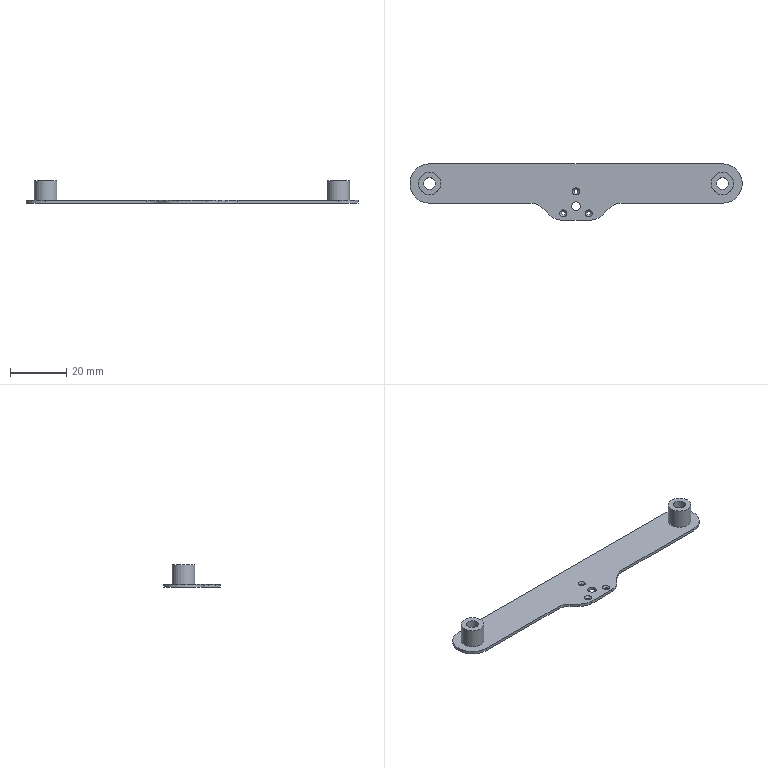Part | NX | features DATUM_CSYS 4, EXTRUDE 4, SKETCH 3, BREP 1, OFFSET_REGION 1, SCALE 1 | 1 solid | 27 faces | box 118 x 20 x 8 mm | volume 2204 mm3 | cylinder 14 | plane 10 | cone 3 | commonest cylinder face diameters 12 x4 1.32 x3 4.2 x2 8 x2 14 x2 3 x1
STEP:
#1=CARTESIAN_POINT('',(1.5,-45.,-19.5));
#2=VERTEX_POINT('',#1);
#3=CARTESIAN_POINT('',(0.,-45.,-19.5));
#4=DIRECTION('',(0.,0.,1.));
#5=DIRECTION('',(1.,0.,0.));
#6=AXIS2_PLACEMENT_3D('',#3,#4,#5);
#7=CIRCLE('',#6,1.5);
#8=EDGE_CURVE('',#2,#2,#7,.T.);
#9=ORIENTED_EDGE('',*,*,#8,.T.);
#10=EDGE_LOOP('',(#9));
#11=FACE_BOUND('',#10,.T.);
#12=CARTESIAN_POINT('',(1.5,-45.,-20.5));
#13=VERTEX_POINT('',#12);
#14=CARTESIAN_POINT('',(0.,-45.,-20.5));
#15=DIRECTION('',(0.,0.,1.));
#16=DIRECTION('',(1.,0.,0.));
#17=AXIS2_PLACEMENT_3D('',#14,#15,#16);
#18=CIRCLE('',#17,1.5);
#19=EDGE_CURVE('',#13,#13,#18,.T.);
#20=ORIENTED_EDGE('',*,*,#19,.F.);
#21=EDGE_LOOP('',(#20));
#22=FACE_BOUND('',#21,.T.);
#23=CARTESIAN_POINT('',(0.,-45.,-19.5));
#24=DIRECTION('',(0.,0.,1.));
#25=DIRECTION('',(1.,0.,0.));
#26=AXIS2_PLACEMENT_3D('',#23,#24,#25);
#27=CYLINDRICAL_SURFACE('',#26,1.5);
#28=ADVANCED_FACE('',(#11,#22),#27,.F.);
#29=CARTESIAN_POINT('',(1.26,-39.8,-19.5));
#30=VERTEX_POINT('',#29);
#31=CARTESIAN_POINT('',(0.,-39.8,-19.5));
#32=DIRECTION('',(0.,0.,1.));
#33=DIRECTION('',(1.,0.,0.));
#34=AXIS2_PLACEMENT_3D('',#31,#32,#33);
#35=CIRCLE('',#34,1.26);
#36=EDGE_CURVE('',#30,#30,#35,.T.);
#37=ORIENTED_EDGE('',*,*,#36,.T.);
#38=EDGE_LOOP('',(#37));
#39=FACE_BOUND('',#38,.T.);
#40=CARTESIAN_POINT('',(0.66,-39.8,-20.1));
#41=VERTEX_POINT('',#40);
#42=CARTESIAN_POINT('',(0.,-39.8,-20.1));
#43=DIRECTION('',(0.,0.,1.));
#44=DIRECTION('',(1.,0.,0.));
#45=AXIS2_PLACEMENT_3D('',#42,#43,#44);
#46=CIRCLE('',#45,0.66);
#47=EDGE_CURVE('',#41,#41,#46,.T.);
#48=ORIENTED_EDGE('',*,*,#47,.F.);
#49=EDGE_LOOP('',(#48));
#50=FACE_BOUND('',#49,.T.);
#51=CARTESIAN_POINT('',(0.,-39.8,-19.5));
#52=DIRECTION('',(0.,0.,1.));
#53=DIRECTION('',(1.,0.,0.));
#54=AXIS2_PLACEMENT_3D('',#51,#52,#53);
#55=CONICAL_SURFACE('',#54,1.26,0.7854);
#56=ADVANCED_FACE('',(#39,#50),#55,.F.);
#57=ORIENTED_EDGE('',*,*,#47,.T.);
#58=EDGE_LOOP('',(#57));
#59=FACE_BOUND('',#58,.T.);
#60=CARTESIAN_POINT('',(0.66,-39.8,-20.5));
#61=VERTEX_POINT('',#60);
#62=CARTESIAN_POINT('',(0.,-39.8,-20.5));
#63=DIRECTION('',(0.,0.,1.));
#64=DIRECTION('',(1.,0.,0.));
#65=AXIS2_PLACEMENT_3D('',#62,#63,#64);
#66=CIRCLE('',#65,0.66);
#67=EDGE_CURVE('',#61,#61,#66,.T.);
#68=ORIENTED_EDGE('',*,*,#67,.F.);
#69=EDGE_LOOP('',(#68));
#70=FACE_BOUND('',#69,.T.);
#71=CARTESIAN_POINT('',(0.,-39.8,-19.5));
#72=DIRECTION('',(0.,0.,1.));
#73=DIRECTION('',(1.,0.,0.));
#74=AXIS2_PLACEMENT_3D('',#71,#72,#73);
#75=CYLINDRICAL_SURFACE('',#74,0.66);
#76=ADVANCED_FACE('',(#59,#70),#75,.F.);
#77=CARTESIAN_POINT('',(-3.243,-47.6,-19.5));
#78=VERTEX_POINT('',#77);
#79=CARTESIAN_POINT('',(-4.503,-47.6,-19.5));
#80=DIRECTION('',(0.,0.,1.));
#81=DIRECTION('',(1.,0.,0.));
#82=AXIS2_PLACEMENT_3D('',#79,#80,#81);
#83=CIRCLE('',#82,1.26);
#84=EDGE_CURVE('',#78,#78,#83,.T.);
#85=ORIENTED_EDGE('',*,*,#84,.T.);
#86=EDGE_LOOP('',(#85));
#87=FACE_BOUND('',#86,.T.);
#88=CARTESIAN_POINT('',(-3.843,-47.6,-20.1));
#89=VERTEX_POINT('',#88);
#90=CARTESIAN_POINT('',(-4.503,-47.6,-20.1));
#91=DIRECTION('',(0.,0.,1.));
#92=DIRECTION('',(1.,0.,0.));
#93=AXIS2_PLACEMENT_3D('',#90,#91,#92);
#94=CIRCLE('',#93,0.66);
#95=EDGE_CURVE('',#89,#89,#94,.T.);
#96=ORIENTED_EDGE('',*,*,#95,.F.);
#97=EDGE_LOOP('',(#96));
#98=FACE_BOUND('',#97,.T.);
#99=CARTESIAN_POINT('',(-4.503,-47.6,-19.5));
#100=DIRECTION('',(0.,0.,1.));
#101=DIRECTION('',(1.,0.,0.));
#102=AXIS2_PLACEMENT_3D('',#99,#100,#101);
#103=CONICAL_SURFACE('',#102,1.26,0.7854);
#104=ADVANCED_FACE('',(#87,#98),#103,.F.);
#105=ORIENTED_EDGE('',*,*,#95,.T.);
#106=EDGE_LOOP('',(#105));
#107=FACE_BOUND('',#106,.T.);
#108=CARTESIAN_POINT('',(-3.843,-47.6,-20.5));
#109=VERTEX_POINT('',#108);
#110=CARTESIAN_POINT('',(-4.503,-47.6,-20.5));
#111=DIRECTION('',(0.,0.,1.));
#112=DIRECTION('',(1.,0.,0.));
#113=AXIS2_PLACEMENT_3D('',#110,#111,#112);
#114=CIRCLE('',#113,0.66);
#115=EDGE_CURVE('',#109,#109,#114,.T.);
#116=ORIENTED_EDGE('',*,*,#115,.F.);
#117=EDGE_LOOP('',(#116));
#118=FACE_BOUND('',#117,.T.);
#119=CARTESIAN_POINT('',(-4.503,-47.6,-19.5));
#120=DIRECTION('',(0.,0.,1.));
#121=DIRECTION('',(1.,0.,0.));
#122=AXIS2_PLACEMENT_3D('',#119,#120,#121);
#123=CYLINDRICAL_SURFACE('',#122,0.66);
#124=ADVANCED_FACE('',(#107,#118),#123,.F.);
#125=CARTESIAN_POINT('',(5.763,-47.6,-19.5));
#126=VERTEX_POINT('',#125);
#127=CARTESIAN_POINT('',(4.503,-47.6,-19.5));
#128=DIRECTION('',(0.,0.,1.));
#129=DIRECTION('',(1.,0.,0.));
#130=AXIS2_PLACEMENT_3D('',#127,#128,#129);
#131=CIRCLE('',#130,1.26);
#132=EDGE_CURVE('',#126,#126,#131,.T.);
#133=ORIENTED_EDGE('',*,*,#132,.T.);
#134=EDGE_LOOP('',(#133));
#135=FACE_BOUND('',#134,.T.);
#136=CARTESIAN_POINT('',(5.163,-47.6,-20.1));
#137=VERTEX_POINT('',#136);
#138=CARTESIAN_POINT('',(4.503,-47.6,-20.1));
#139=DIRECTION('',(0.,0.,1.));
#140=DIRECTION('',(1.,0.,0.));
#141=AXIS2_PLACEMENT_3D('',#138,#139,#140);
#142=CIRCLE('',#141,0.66);
#143=EDGE_CURVE('',#137,#137,#142,.T.);
#144=ORIENTED_EDGE('',*,*,#143,.F.);
#145=EDGE_LOOP('',(#144));
#146=FACE_BOUND('',#145,.T.);
#147=CARTESIAN_POINT('',(4.503,-47.6,-19.5));
#148=DIRECTION('',(0.,0.,1.));
#149=DIRECTION('',(1.,0.,0.));
#150=AXIS2_PLACEMENT_3D('',#147,#148,#149);
#151=CONICAL_SURFACE('',#150,1.26,0.7854);
#152=ADVANCED_FACE('',(#135,#146),#151,.F.);
#153=ORIENTED_EDGE('',*,*,#143,.T.);
#154=EDGE_LOOP('',(#153));
#155=FACE_BOUND('',#154,.T.);
#156=CARTESIAN_POINT('',(5.163,-47.6,-20.5));
#157=VERTEX_POINT('',#156);
#158=CARTESIAN_POINT('',(4.503,-47.6,-20.5));
#159=DIRECTION('',(0.,0.,1.));
#160=DIRECTION('',(1.,0.,0.));
#161=AXIS2_PLACEMENT_3D('',#158,#159,#160);
#162=CIRCLE('',#161,0.66);
#163=EDGE_CURVE('',#157,#157,#162,.T.);
#164=ORIENTED_EDGE('',*,*,#163,.F.);
#165=EDGE_LOOP('',(#164));
#166=FACE_BOUND('',#165,.T.);
#167=CARTESIAN_POINT('',(4.503,-47.6,-19.5));
#168=DIRECTION('',(0.,0.,1.));
#169=DIRECTION('',(1.,0.,0.));
#170=AXIS2_PLACEMENT_3D('',#167,#168,#169);
#171=CYLINDRICAL_SURFACE('',#170,0.66);
#172=ADVANCED_FACE('',(#155,#166),#171,.F.);
#173=CARTESIAN_POINT('',(-52.,-30.,-19.5));
#174=VERTEX_POINT('',#173);
#175=CARTESIAN_POINT('',(-52.,-44.,-19.5));
#176=VERTEX_POINT('',#175);
#177=CARTESIAN_POINT('',(-52.,-37.,-19.5));
#178=DIRECTION('',(0.,0.,1.));
#179=DIRECTION('',(1.,0.,0.));
#180=AXIS2_PLACEMENT_3D('',#177,#178,#179);
#181=CIRCLE('',#180,7.);
#182=EDGE_CURVE('',#174,#176,#181,.T.);
#183=ORIENTED_EDGE('',*,*,#182,.F.);
#184=CARTESIAN_POINT('',(-52.,-30.,-20.5));
#185=VERTEX_POINT('',#184);
#186=CARTESIAN_POINT('',(-52.,-30.,-19.5));
#187=DIRECTION('',(0.,0.,1.));
#188=VECTOR('',#187,1000.);
#189=LINE('',#186,#188);
#190=EDGE_CURVE('',#185,#174,#189,.T.);
#191=ORIENTED_EDGE('',*,*,#190,.F.);
#192=CARTESIAN_POINT('',(-52.,-44.,-20.5));
#193=VERTEX_POINT('',#192);
#194=CARTESIAN_POINT('',(-52.,-37.,-20.5));
#195=DIRECTION('',(0.,0.,-1.));
#196=DIRECTION('',(1.,0.,0.));
#197=AXIS2_PLACEMENT_3D('',#194,#195,#196);
#198=CIRCLE('',#197,7.);
#199=EDGE_CURVE('',#193,#185,#198,.T.);
#200=ORIENTED_EDGE('',*,*,#199,.F.);
#201=CARTESIAN_POINT('',(-52.,-44.,-19.5));
#202=DIRECTION('',(0.,0.,-1.));
#203=VECTOR('',#202,1000.);
#204=LINE('',#201,#203);
#205=EDGE_CURVE('',#176,#193,#204,.T.);
#206=ORIENTED_EDGE('',*,*,#205,.F.);
#207=EDGE_LOOP('',(#183,#191,#200,#206));
#208=FACE_BOUND('',#207,.T.);
#209=CARTESIAN_POINT('',(-52.,-37.,-19.5));
#210=DIRECTION('',(0.,0.,-1.));
#211=DIRECTION('',(-1.,0.,0.));
#212=AXIS2_PLACEMENT_3D('',#209,#210,#211);
#213=CYLINDRICAL_SURFACE('',#212,7.);
#214=ADVANCED_FACE('',(#208),#213,.T.);
#215=ORIENTED_EDGE('',*,*,#190,.T.);
#216=CARTESIAN_POINT('',(52.,-30.,-19.5));
#217=VERTEX_POINT('',#216);
#218=CARTESIAN_POINT('',(-59.,-30.,-19.5));
#219=DIRECTION('',(-1.,0.,0.));
#220=VECTOR('',#219,1000.);
#221=LINE('',#218,#220);
#222=EDGE_CURVE('',#217,#174,#221,.T.);
#223=ORIENTED_EDGE('',*,*,#222,.F.);
#224=CARTESIAN_POINT('',(52.,-30.,-20.5));
#225=VERTEX_POINT('',#224);
#226=CARTESIAN_POINT('',(52.,-30.,-19.5));
#227=DIRECTION('',(0.,0.,-1.));
#228=VECTOR('',#227,1000.);
#229=LINE('',#226,#228);
#230=EDGE_CURVE('',#217,#225,#229,.T.);
#231=ORIENTED_EDGE('',*,*,#230,.T.);
#232=CARTESIAN_POINT('',(-59.,-30.,-20.5));
#233=DIRECTION('',(-1.,0.,0.));
#234=VECTOR('',#233,1000.);
#235=LINE('',#232,#234);
#236=EDGE_CURVE('',#225,#185,#235,.T.);
#237=ORIENTED_EDGE('',*,*,#236,.T.);
#238=EDGE_LOOP('',(#215,#223,#231,#237));
#239=FACE_BOUND('',#238,.T.);
#240=CARTESIAN_POINT('',(-59.,-30.,-19.5));
#241=DIRECTION('',(0.,-1.,0.));
#242=DIRECTION('',(0.,0.,-1.));
#243=AXIS2_PLACEMENT_3D('',#240,#241,#242);
#244=PLANE('',#243);
#245=ADVANCED_FACE('',(#239),#244,.F.);
#246=ORIENTED_EDGE('',*,*,#230,.F.);
#247=CARTESIAN_POINT('',(52.,-44.,-19.5));
#248=VERTEX_POINT('',#247);
#249=CARTESIAN_POINT('',(52.,-37.,-19.5));
#250=DIRECTION('',(0.,0.,1.));
#251=DIRECTION('',(1.,0.,0.));
#252=AXIS2_PLACEMENT_3D('',#249,#250,#251);
#253=CIRCLE('',#252,7.);
#254=EDGE_CURVE('',#248,#217,#253,.T.);
#255=ORIENTED_EDGE('',*,*,#254,.F.);
#256=CARTESIAN_POINT('',(52.,-44.,-20.5));
#257=VERTEX_POINT('',#256);
#258=CARTESIAN_POINT('',(52.,-44.,-19.5));
#259=DIRECTION('',(0.,0.,1.));
#260=VECTOR('',#259,1000.);
#261=LINE('',#258,#260);
#262=EDGE_CURVE('',#257,#248,#261,.T.);
#263=ORIENTED_EDGE('',*,*,#262,.F.);
#264=CARTESIAN_POINT('',(52.,-37.,-20.5));
#265=DIRECTION('',(0.,0.,-1.));
#266=DIRECTION('',(1.,0.,0.));
#267=AXIS2_PLACEMENT_3D('',#264,#265,#266);
#268=CIRCLE('',#267,7.);
#269=EDGE_CURVE('',#225,#257,#268,.T.);
#270=ORIENTED_EDGE('',*,*,#269,.F.);
#271=EDGE_LOOP('',(#246,#255,#263,#270));
#272=FACE_BOUND('',#271,.T.);
#273=CARTESIAN_POINT('',(52.,-37.,-19.5));
#274=DIRECTION('',(0.,0.,-1.));
#275=DIRECTION('',(-1.,0.,0.));
#276=AXIS2_PLACEMENT_3D('',#273,#274,#275);
#277=CYLINDRICAL_SURFACE('',#276,7.);
#278=ADVANCED_FACE('',(#272),#277,.T.);
#279=CARTESIAN_POINT('',(-15.985,-44.,-20.5));
#280=VERTEX_POINT('',#279);
#281=CARTESIAN_POINT('',(-59.,-44.,-20.5));
#282=DIRECTION('',(1.,0.,0.));
#283=VECTOR('',#282,1000.);
#284=LINE('',#281,#283);
#285=EDGE_CURVE('',#193,#280,#284,.T.);
#286=ORIENTED_EDGE('',*,*,#285,.T.);
#287=CARTESIAN_POINT('',(-15.985,-44.,-19.5));
#288=VERTEX_POINT('',#287);
#289=CARTESIAN_POINT('',(-15.985,-44.,-19.5));
#290=DIRECTION('',(0.,0.,1.));
#291=VECTOR('',#290,1000.);
#292=LINE('',#289,#291);
#293=EDGE_CURVE('',#280,#288,#292,.T.);
#294=ORIENTED_EDGE('',*,*,#293,.T.);
#295=CARTESIAN_POINT('',(-59.,-44.,-19.5));
#296=DIRECTION('',(1.,0.,0.));
#297=VECTOR('',#296,1000.);
#298=LINE('',#295,#297);
#299=EDGE_CURVE('',#176,#288,#298,.T.);
#300=ORIENTED_EDGE('',*,*,#299,.F.);
#301=ORIENTED_EDGE('',*,*,#205,.T.);
#302=EDGE_LOOP('',(#286,#294,#300,#301));
#303=FACE_BOUND('',#302,.T.);
#304=CARTESIAN_POINT('',(-59.,-44.,-19.5));
#305=DIRECTION('',(0.,1.,0.));
#306=DIRECTION('',(0.,0.,1.));
#307=AXIS2_PLACEMENT_3D('',#304,#305,#306);
#308=PLANE('',#307);
#309=ADVANCED_FACE('',(#303),#308,.F.);
#310=CARTESIAN_POINT('',(15.985,-44.,-19.5));
#311=VERTEX_POINT('',#310);
#312=CARTESIAN_POINT('',(-59.,-44.,-19.5));
#313=DIRECTION('',(1.,0.,0.));
#314=VECTOR('',#313,1000.);
#315=LINE('',#312,#314);
#316=EDGE_CURVE('',#311,#248,#315,.T.);
#317=ORIENTED_EDGE('',*,*,#316,.F.);
#318=CARTESIAN_POINT('',(15.985,-44.,-20.5));
#319=VERTEX_POINT('',#318);
#320=CARTESIAN_POINT('',(15.985,-44.,-19.5));
#321=DIRECTION('',(0.,0.,-1.));
#322=VECTOR('',#321,1000.);
#323=LINE('',#320,#322);
#324=EDGE_CURVE('',#311,#319,#323,.T.);
#325=ORIENTED_EDGE('',*,*,#324,.T.);
#326=CARTESIAN_POINT('',(-59.,-44.,-20.5));
#327=DIRECTION('',(1.,0.,0.));
#328=VECTOR('',#327,1000.);
#329=LINE('',#326,#328);
#330=EDGE_CURVE('',#319,#257,#329,.T.);
#331=ORIENTED_EDGE('',*,*,#330,.T.);
#332=ORIENTED_EDGE('',*,*,#262,.T.);
#333=EDGE_LOOP('',(#317,#325,#331,#332));
#334=FACE_BOUND('',#333,.T.);
#335=CARTESIAN_POINT('',(-59.,-44.,-19.5));
#336=DIRECTION('',(0.,1.,0.));
#337=DIRECTION('',(0.,0.,1.));
#338=AXIS2_PLACEMENT_3D('',#335,#336,#337);
#339=PLANE('',#338);
#340=ADVANCED_FACE('',(#334),#339,.F.);
#341=CARTESIAN_POINT('',(-48.,-37.,-19.5));
#342=VERTEX_POINT('',#341);
#343=CARTESIAN_POINT('',(-52.,-37.,-19.5));
#344=DIRECTION('',(0.,0.,1.));
#345=DIRECTION('',(1.,0.,0.));
#346=AXIS2_PLACEMENT_3D('',#343,#344,#345);
#347=CIRCLE('',#346,4.);
#348=EDGE_CURVE('',#342,#342,#347,.T.);
#349=ORIENTED_EDGE('',*,*,#348,.F.);
#350=EDGE_LOOP('',(#349));
#351=FACE_BOUND('',#350,.T.);
#352=CARTESIAN_POINT('',(56.,-37.,-19.5));
#353=VERTEX_POINT('',#352);
#354=CARTESIAN_POINT('',(52.,-37.,-19.5));
#355=DIRECTION('',(0.,0.,1.));
#356=DIRECTION('',(1.,0.,0.));
#357=AXIS2_PLACEMENT_3D('',#354,#355,#356);
#358=CIRCLE('',#357,4.);
#359=EDGE_CURVE('',#353,#353,#358,.T.);
#360=ORIENTED_EDGE('',*,*,#359,.F.);
#361=EDGE_LOOP('',(#360));
#362=FACE_BOUND('',#361,.T.);
#363=ORIENTED_EDGE('',*,*,#222,.T.);
#364=ORIENTED_EDGE('',*,*,#182,.T.);
#365=ORIENTED_EDGE('',*,*,#299,.T.);
#366=CARTESIAN_POINT('',(-11.743,-45.757,-19.5));
#367=VERTEX_POINT('',#366);
#368=CARTESIAN_POINT('',(-15.985,-50.,-19.5));
#369=DIRECTION('',(0.,0.,-1.));
#370=DIRECTION('',(1.,0.,0.));
#371=AXIS2_PLACEMENT_3D('',#368,#369,#370);
#372=CIRCLE('',#371,6.);
#373=EDGE_CURVE('',#288,#367,#372,.T.);
#374=ORIENTED_EDGE('',*,*,#373,.T.);
#375=CARTESIAN_POINT('',(-9.257,-48.243,-19.5));
#376=VERTEX_POINT('',#375);
#377=CARTESIAN_POINT('',(-10.25,-47.25,-19.5));
#378=DIRECTION('',(-0.7071,0.7071,0.));
#379=VECTOR('',#378,1000.);
#380=LINE('',#377,#379);
#381=EDGE_CURVE('',#376,#367,#380,.T.);
#382=ORIENTED_EDGE('',*,*,#381,.F.);
#383=CARTESIAN_POINT('',(-5.015,-50.,-19.5));
#384=VERTEX_POINT('',#383);
#385=CARTESIAN_POINT('',(-5.015,-44.,-19.5));
#386=DIRECTION('',(0.,0.,1.));
#387=DIRECTION('',(1.,0.,0.));
#388=AXIS2_PLACEMENT_3D('',#385,#386,#387);
#389=CIRCLE('',#388,6.);
#390=EDGE_CURVE('',#376,#384,#389,.T.);
#391=ORIENTED_EDGE('',*,*,#390,.T.);
#392=CARTESIAN_POINT('',(5.015,-50.,-19.5));
#393=VERTEX_POINT('',#392);
#394=CARTESIAN_POINT('',(0.,-50.,-19.5));
#395=DIRECTION('',(-1.,0.,0.));
#396=VECTOR('',#395,1000.);
#397=LINE('',#394,#396);
#398=EDGE_CURVE('',#393,#384,#397,.T.);
#399=ORIENTED_EDGE('',*,*,#398,.F.);
#400=CARTESIAN_POINT('',(9.257,-48.243,-19.5));
#401=VERTEX_POINT('',#400);
#402=CARTESIAN_POINT('',(5.015,-44.,-19.5));
#403=DIRECTION('',(0.,0.,1.));
#404=DIRECTION('',(1.,0.,0.));
#405=AXIS2_PLACEMENT_3D('',#402,#403,#404);
#406=CIRCLE('',#405,6.);
#407=EDGE_CURVE('',#393,#401,#406,.T.);
#408=ORIENTED_EDGE('',*,*,#407,.T.);
#409=CARTESIAN_POINT('',(11.743,-45.757,-19.5));
#410=VERTEX_POINT('',#409);
#411=CARTESIAN_POINT('',(10.25,-47.25,-19.5));
#412=DIRECTION('',(-0.7071,-0.7071,0.));
#413=VECTOR('',#412,1000.);
#414=LINE('',#411,#413);
#415=EDGE_CURVE('',#410,#401,#414,.T.);
#416=ORIENTED_EDGE('',*,*,#415,.F.);
#417=CARTESIAN_POINT('',(15.985,-50.,-19.5));
#418=DIRECTION('',(0.,0.,-1.));
#419=DIRECTION('',(1.,0.,0.));
#420=AXIS2_PLACEMENT_3D('',#417,#418,#419);
#421=CIRCLE('',#420,6.);
#422=EDGE_CURVE('',#410,#311,#421,.T.);
#423=ORIENTED_EDGE('',*,*,#422,.T.);
#424=ORIENTED_EDGE('',*,*,#316,.T.);
#425=ORIENTED_EDGE('',*,*,#254,.T.);
#426=EDGE_LOOP('',(#363,#364,#365,#374,#382,#391,#399,#408,#416,#423,#424,#425));
#427=FACE_BOUND('',#426,.T.);
#428=ORIENTED_EDGE('',*,*,#8,.F.);
#429=EDGE_LOOP('',(#428));
#430=FACE_BOUND('',#429,.T.);
#431=ORIENTED_EDGE('',*,*,#36,.F.);
#432=EDGE_LOOP('',(#431));
#433=FACE_BOUND('',#432,.T.);
#434=ORIENTED_EDGE('',*,*,#84,.F.);
#435=EDGE_LOOP('',(#434));
#436=FACE_BOUND('',#435,.T.);
#437=ORIENTED_EDGE('',*,*,#132,.F.);
#438=EDGE_LOOP('',(#437));
#439=FACE_BOUND('',#438,.T.);
#440=CARTESIAN_POINT('',(0.,-37.,-19.5));
#441=DIRECTION('',(0.,0.,1.));
#442=DIRECTION('',(1.,0.,0.));
#443=AXIS2_PLACEMENT_3D('',#440,#441,#442);
#444=PLANE('',#443);
#445=ADVANCED_FACE('',(#351,#362,#427,#430,#433,#436,#439),#444,.T.);
#446=CARTESIAN_POINT('',(54.1,-37.,-20.5));
#447=VERTEX_POINT('',#446);
#448=CARTESIAN_POINT('',(52.,-37.,-20.5));
#449=DIRECTION('',(0.,0.,1.));
#450=DIRECTION('',(1.,0.,0.));
#451=AXIS2_PLACEMENT_3D('',#448,#449,#450);
#452=CIRCLE('',#451,2.1);
#453=EDGE_CURVE('',#447,#447,#452,.F.);
#454=ORIENTED_EDGE('',*,*,#453,.F.);
#455=EDGE_LOOP('',(#454));
#456=FACE_BOUND('',#455,.T.);
#457=CARTESIAN_POINT('',(-49.9,-37.,-20.5));
#458=VERTEX_POINT('',#457);
#459=CARTESIAN_POINT('',(-52.,-37.,-20.5));
#460=DIRECTION('',(0.,0.,1.));
#461=DIRECTION('',(1.,0.,0.));
#462=AXIS2_PLACEMENT_3D('',#459,#460,#461);
#463=CIRCLE('',#462,2.1);
#464=EDGE_CURVE('',#458,#458,#463,.F.);
#465=ORIENTED_EDGE('',*,*,#464,.F.);
#466=EDGE_LOOP('',(#465));
#467=FACE_BOUND('',#466,.T.);
#468=ORIENTED_EDGE('',*,*,#199,.T.);
#469=ORIENTED_EDGE('',*,*,#236,.F.);
#470=ORIENTED_EDGE('',*,*,#269,.T.);
#471=ORIENTED_EDGE('',*,*,#330,.F.);
#472=CARTESIAN_POINT('',(11.743,-45.757,-20.5));
#473=VERTEX_POINT('',#472);
#474=CARTESIAN_POINT('',(15.985,-50.,-20.5));
#475=DIRECTION('',(0.,0.,1.));
#476=DIRECTION('',(1.,0.,0.));
#477=AXIS2_PLACEMENT_3D('',#474,#475,#476);
#478=CIRCLE('',#477,6.);
#479=EDGE_CURVE('',#319,#473,#478,.T.);
#480=ORIENTED_EDGE('',*,*,#479,.T.);
#481=CARTESIAN_POINT('',(9.257,-48.243,-20.5));
#482=VERTEX_POINT('',#481);
#483=CARTESIAN_POINT('',(10.25,-47.25,-20.5));
#484=DIRECTION('',(-0.7071,-0.7071,0.));
#485=VECTOR('',#484,1000.);
#486=LINE('',#483,#485);
#487=EDGE_CURVE('',#473,#482,#486,.T.);
#488=ORIENTED_EDGE('',*,*,#487,.T.);
#489=CARTESIAN_POINT('',(5.015,-50.,-20.5));
#490=VERTEX_POINT('',#489);
#491=CARTESIAN_POINT('',(5.015,-44.,-20.5));
#492=DIRECTION('',(0.,0.,-1.));
#493=DIRECTION('',(1.,0.,0.));
#494=AXIS2_PLACEMENT_3D('',#491,#492,#493);
#495=CIRCLE('',#494,6.);
#496=EDGE_CURVE('',#482,#490,#495,.T.);
#497=ORIENTED_EDGE('',*,*,#496,.T.);
#498=CARTESIAN_POINT('',(-5.015,-50.,-20.5));
#499=VERTEX_POINT('',#498);
#500=CARTESIAN_POINT('',(0.,-50.,-20.5));
#501=DIRECTION('',(-1.,0.,0.));
#502=VECTOR('',#501,1000.);
#503=LINE('',#500,#502);
#504=EDGE_CURVE('',#490,#499,#503,.T.);
#505=ORIENTED_EDGE('',*,*,#504,.T.);
#506=CARTESIAN_POINT('',(-9.257,-48.243,-20.5));
#507=VERTEX_POINT('',#506);
#508=CARTESIAN_POINT('',(-5.015,-44.,-20.5));
#509=DIRECTION('',(0.,0.,-1.));
#510=DIRECTION('',(1.,0.,0.));
#511=AXIS2_PLACEMENT_3D('',#508,#509,#510);
#512=CIRCLE('',#511,6.);
#513=EDGE_CURVE('',#499,#507,#512,.T.);
#514=ORIENTED_EDGE('',*,*,#513,.T.);
#515=CARTESIAN_POINT('',(-11.743,-45.757,-20.5));
#516=VERTEX_POINT('',#515);
#517=CARTESIAN_POINT('',(-10.25,-47.25,-20.5));
#518=DIRECTION('',(-0.7071,0.7071,0.));
#519=VECTOR('',#518,1000.);
#520=LINE('',#517,#519);
#521=EDGE_CURVE('',#507,#516,#520,.T.);
#522=ORIENTED_EDGE('',*,*,#521,.T.);
#523=CARTESIAN_POINT('',(-15.985,-50.,-20.5));
#524=DIRECTION('',(0.,0.,1.));
#525=DIRECTION('',(1.,0.,0.));
#526=AXIS2_PLACEMENT_3D('',#523,#524,#525);
#527=CIRCLE('',#526,6.);
#528=EDGE_CURVE('',#516,#280,#527,.T.);
#529=ORIENTED_EDGE('',*,*,#528,.T.);
#530=ORIENTED_EDGE('',*,*,#285,.F.);
#531=EDGE_LOOP('',(#468,#469,#470,#471,#480,#488,#497,#505,#514,#522,#529,#530));
#532=FACE_BOUND('',#531,.T.);
#533=ORIENTED_EDGE('',*,*,#163,.T.);
#534=EDGE_LOOP('',(#533));
#535=FACE_BOUND('',#534,.T.);
#536=ORIENTED_EDGE('',*,*,#115,.T.);
#537=EDGE_LOOP('',(#536));
#538=FACE_BOUND('',#537,.T.);
#539=ORIENTED_EDGE('',*,*,#67,.T.);
#540=EDGE_LOOP('',(#539));
#541=FACE_BOUND('',#540,.T.);
#542=ORIENTED_EDGE('',*,*,#19,.T.);
#543=EDGE_LOOP('',(#542));
#544=FACE_BOUND('',#543,.T.);
#545=CARTESIAN_POINT('',(0.,-37.,-20.5));
#546=DIRECTION('',(0.,0.,1.));
#547=DIRECTION('',(1.,0.,0.));
#548=AXIS2_PLACEMENT_3D('',#545,#546,#547);
#549=PLANE('',#548);
#550=ADVANCED_FACE('',(#456,#467,#532,#535,#538,#541,#544),#549,.F.);
#551=ORIENTED_EDGE('',*,*,#381,.T.);
#552=CARTESIAN_POINT('',(-11.743,-45.757,8.159));
#553=DIRECTION('',(0.,0.,-1.));
#554=VECTOR('',#553,1000.);
#555=LINE('',#552,#554);
#556=EDGE_CURVE('',#367,#516,#555,.T.);
#557=ORIENTED_EDGE('',*,*,#556,.T.);
#558=ORIENTED_EDGE('',*,*,#521,.F.);
#559=CARTESIAN_POINT('',(-9.257,-48.243,8.159));
#560=DIRECTION('',(0.,0.,1.));
#561=VECTOR('',#560,1000.);
#562=LINE('',#559,#561);
#563=EDGE_CURVE('',#507,#376,#562,.T.);
#564=ORIENTED_EDGE('',*,*,#563,.T.);
#565=EDGE_LOOP('',(#551,#557,#558,#564));
#566=FACE_BOUND('',#565,.T.);
#567=CARTESIAN_POINT('',(-10.25,-47.25,8.159));
#568=DIRECTION('',(-0.7071,-0.7071,0.));
#569=DIRECTION('',(0.7071,-0.7071,0.));
#570=AXIS2_PLACEMENT_3D('',#567,#568,#569);
#571=PLANE('',#570);
#572=ADVANCED_FACE('',(#566),#571,.T.);
#573=ORIENTED_EDGE('',*,*,#487,.F.);
#574=CARTESIAN_POINT('',(11.743,-45.757,8.159));
#575=DIRECTION('',(0.,0.,1.));
#576=VECTOR('',#575,1000.);
#577=LINE('',#574,#576);
#578=EDGE_CURVE('',#473,#410,#577,.T.);
#579=ORIENTED_EDGE('',*,*,#578,.T.);
#580=ORIENTED_EDGE('',*,*,#415,.T.);
#581=CARTESIAN_POINT('',(9.257,-48.243,8.159));
#582=DIRECTION('',(0.,0.,-1.));
#583=VECTOR('',#582,1000.);
#584=LINE('',#581,#583);
#585=EDGE_CURVE('',#401,#482,#584,.T.);
#586=ORIENTED_EDGE('',*,*,#585,.T.);
#587=EDGE_LOOP('',(#573,#579,#580,#586));
#588=FACE_BOUND('',#587,.T.);
#589=CARTESIAN_POINT('',(10.25,-47.25,8.159));
#590=DIRECTION('',(0.7071,-0.7071,0.));
#591=DIRECTION('',(0.7071,0.7071,0.));
#592=AXIS2_PLACEMENT_3D('',#589,#590,#591);
#593=PLANE('',#592);
#594=ADVANCED_FACE('',(#588),#593,.T.);
#595=ORIENTED_EDGE('',*,*,#504,.F.);
#596=CARTESIAN_POINT('',(5.015,-50.,8.159));
#597=DIRECTION('',(0.,0.,1.));
#598=VECTOR('',#597,1000.);
#599=LINE('',#596,#598);
#600=EDGE_CURVE('',#490,#393,#599,.T.);
#601=ORIENTED_EDGE('',*,*,#600,.T.);
#602=ORIENTED_EDGE('',*,*,#398,.T.);
#603=CARTESIAN_POINT('',(-5.015,-50.,8.159));
#604=DIRECTION('',(0.,0.,-1.));
#605=VECTOR('',#604,1000.);
#606=LINE('',#603,#605);
#607=EDGE_CURVE('',#384,#499,#606,.T.);
#608=ORIENTED_EDGE('',*,*,#607,.T.);
#609=EDGE_LOOP('',(#595,#601,#602,#608));
#610=FACE_BOUND('',#609,.T.);
#611=CARTESIAN_POINT('',(0.,-50.,8.159));
#612=DIRECTION('',(0.,-1.,0.));
#613=DIRECTION('',(0.,0.,-1.));
#614=AXIS2_PLACEMENT_3D('',#611,#612,#613);
#615=PLANE('',#614);
#616=ADVANCED_FACE('',(#610),#615,.T.);
#617=ORIENTED_EDGE('',*,*,#373,.F.);
#618=ORIENTED_EDGE('',*,*,#293,.F.);
#619=ORIENTED_EDGE('',*,*,#528,.F.);
#620=ORIENTED_EDGE('',*,*,#556,.F.);
#621=EDGE_LOOP('',(#617,#618,#619,#620));
#622=FACE_BOUND('',#621,.T.);
#623=CARTESIAN_POINT('',(-15.985,-50.,8.159));
#624=DIRECTION('',(0.,0.,-1.));
#625=DIRECTION('',(-1.,0.,0.));
#626=AXIS2_PLACEMENT_3D('',#623,#624,#625);
#627=CYLINDRICAL_SURFACE('',#626,6.);
#628=ADVANCED_FACE('',(#622),#627,.F.);
#629=ORIENTED_EDGE('',*,*,#422,.F.);
#630=ORIENTED_EDGE('',*,*,#578,.F.);
#631=ORIENTED_EDGE('',*,*,#479,.F.);
#632=ORIENTED_EDGE('',*,*,#324,.F.);
#633=EDGE_LOOP('',(#629,#630,#631,#632));
#634=FACE_BOUND('',#633,.T.);
#635=CARTESIAN_POINT('',(15.985,-50.,-19.5));
#636=DIRECTION('',(0.,0.,-1.));
#637=DIRECTION('',(-1.,0.,0.));
#638=AXIS2_PLACEMENT_3D('',#635,#636,#637);
#639=CYLINDRICAL_SURFACE('',#638,6.);
#640=ADVANCED_FACE('',(#634),#639,.F.);
#641=ORIENTED_EDGE('',*,*,#407,.F.);
#642=ORIENTED_EDGE('',*,*,#600,.F.);
#643=ORIENTED_EDGE('',*,*,#496,.F.);
#644=ORIENTED_EDGE('',*,*,#585,.F.);
#645=EDGE_LOOP('',(#641,#642,#643,#644));
#646=FACE_BOUND('',#645,.T.);
#647=CARTESIAN_POINT('',(5.015,-44.,8.159));
#648=DIRECTION('',(0.,0.,-1.));
#649=DIRECTION('',(-1.,0.,0.));
#650=AXIS2_PLACEMENT_3D('',#647,#648,#649);
#651=CYLINDRICAL_SURFACE('',#650,6.);
#652=ADVANCED_FACE('',(#646),#651,.T.);
#653=ORIENTED_EDGE('',*,*,#390,.F.);
#654=ORIENTED_EDGE('',*,*,#563,.F.);
#655=ORIENTED_EDGE('',*,*,#513,.F.);
#656=ORIENTED_EDGE('',*,*,#607,.F.);
#657=EDGE_LOOP('',(#653,#654,#655,#656));
#658=FACE_BOUND('',#657,.T.);
#659=CARTESIAN_POINT('',(-5.015,-44.,8.159));
#660=DIRECTION('',(0.,0.,-1.));
#661=DIRECTION('',(-1.,0.,0.));
#662=AXIS2_PLACEMENT_3D('',#659,#660,#661);
#663=CYLINDRICAL_SURFACE('',#662,6.);
#664=ADVANCED_FACE('',(#658),#663,.T.);
#665=ORIENTED_EDGE('',*,*,#464,.T.);
#666=EDGE_LOOP('',(#665));
#667=FACE_BOUND('',#666,.T.);
#668=CARTESIAN_POINT('',(-49.9,-37.,-12.5));
#669=VERTEX_POINT('',#668);
#670=CARTESIAN_POINT('',(-52.,-37.,-12.5));
#671=DIRECTION('',(0.,0.,1.));
#672=DIRECTION('',(1.,0.,0.));
#673=AXIS2_PLACEMENT_3D('',#670,#671,#672);
#674=CIRCLE('',#673,2.1);
#675=EDGE_CURVE('',#669,#669,#674,.T.);
#676=ORIENTED_EDGE('',*,*,#675,.T.);
#677=EDGE_LOOP('',(#676));
#678=FACE_BOUND('',#677,.T.);
#679=CARTESIAN_POINT('',(-52.,-37.,-9.5));
#680=DIRECTION('',(0.,0.,-1.));
#681=DIRECTION('',(-1.,0.,0.));
#682=AXIS2_PLACEMENT_3D('',#679,#680,#681);
#683=CYLINDRICAL_SURFACE('',#682,2.1);
#684=ADVANCED_FACE('',(#667,#678),#683,.F.);
#685=ORIENTED_EDGE('',*,*,#453,.T.);
#686=EDGE_LOOP('',(#685));
#687=FACE_BOUND('',#686,.T.);
#688=CARTESIAN_POINT('',(54.1,-37.,-12.5));
#689=VERTEX_POINT('',#688);
#690=CARTESIAN_POINT('',(52.,-37.,-12.5));
#691=DIRECTION('',(0.,0.,1.));
#692=DIRECTION('',(1.,0.,0.));
#693=AXIS2_PLACEMENT_3D('',#690,#691,#692);
#694=CIRCLE('',#693,2.1);
#695=EDGE_CURVE('',#689,#689,#694,.T.);
#696=ORIENTED_EDGE('',*,*,#695,.T.);
#697=EDGE_LOOP('',(#696));
#698=FACE_BOUND('',#697,.T.);
#699=CARTESIAN_POINT('',(52.,-37.,-9.5));
#700=DIRECTION('',(0.,0.,-1.));
#701=DIRECTION('',(-1.,0.,0.));
#702=AXIS2_PLACEMENT_3D('',#699,#700,#701);
#703=CYLINDRICAL_SURFACE('',#702,2.1);
#704=ADVANCED_FACE('',(#687,#698),#703,.F.);
#705=ORIENTED_EDGE('',*,*,#359,.T.);
#706=EDGE_LOOP('',(#705));
#707=FACE_BOUND('',#706,.T.);
#708=CARTESIAN_POINT('',(56.,-37.,-12.5));
#709=VERTEX_POINT('',#708);
#710=CARTESIAN_POINT('',(52.,-37.,-12.5));
#711=DIRECTION('',(0.,0.,1.));
#712=DIRECTION('',(1.,0.,0.));
#713=AXIS2_PLACEMENT_3D('',#710,#711,#712);
#714=CIRCLE('',#713,4.);
#715=EDGE_CURVE('',#709,#709,#714,.T.);
#716=ORIENTED_EDGE('',*,*,#715,.F.);
#717=EDGE_LOOP('',(#716));
#718=FACE_BOUND('',#717,.T.);
#719=CARTESIAN_POINT('',(52.,-37.,-19.5));
#720=DIRECTION('',(0.,0.,1.));
#721=DIRECTION('',(1.,0.,0.));
#722=AXIS2_PLACEMENT_3D('',#719,#720,#721);
#723=CYLINDRICAL_SURFACE('',#722,4.);
#724=ADVANCED_FACE('',(#707,#718),#723,.T.);
#725=ORIENTED_EDGE('',*,*,#715,.T.);
#726=EDGE_LOOP('',(#725));
#727=FACE_BOUND('',#726,.T.);
#728=ORIENTED_EDGE('',*,*,#695,.F.);
#729=EDGE_LOOP('',(#728));
#730=FACE_BOUND('',#729,.T.);
#731=CARTESIAN_POINT('',(52.,-37.,-12.5));
#732=DIRECTION('',(0.,0.,1.));
#733=DIRECTION('',(1.,0.,0.));
#734=AXIS2_PLACEMENT_3D('',#731,#732,#733);
#735=PLANE('',#734);
#736=ADVANCED_FACE('',(#727,#730),#735,.T.);
#737=ORIENTED_EDGE('',*,*,#348,.T.);
#738=EDGE_LOOP('',(#737));
#739=FACE_BOUND('',#738,.T.);
#740=CARTESIAN_POINT('',(-48.,-37.,-12.5));
#741=VERTEX_POINT('',#740);
#742=CARTESIAN_POINT('',(-52.,-37.,-12.5));
#743=DIRECTION('',(0.,0.,1.));
#744=DIRECTION('',(1.,0.,0.));
#745=AXIS2_PLACEMENT_3D('',#742,#743,#744);
#746=CIRCLE('',#745,4.);
#747=EDGE_CURVE('',#741,#741,#746,.T.);
#748=ORIENTED_EDGE('',*,*,#747,.F.);
#749=EDGE_LOOP('',(#748));
#750=FACE_BOUND('',#749,.T.);
#751=CARTESIAN_POINT('',(-52.,-37.,-19.5));
#752=DIRECTION('',(0.,0.,1.));
#753=DIRECTION('',(1.,0.,0.));
#754=AXIS2_PLACEMENT_3D('',#751,#752,#753);
#755=CYLINDRICAL_SURFACE('',#754,4.);
#756=ADVANCED_FACE('',(#739,#750),#755,.T.);
#757=ORIENTED_EDGE('',*,*,#747,.T.);
#758=EDGE_LOOP('',(#757));
#759=FACE_BOUND('',#758,.T.);
#760=ORIENTED_EDGE('',*,*,#675,.F.);
#761=EDGE_LOOP('',(#760));
#762=FACE_BOUND('',#761,.T.);
#763=CARTESIAN_POINT('',(-52.,-37.,-12.5));
#764=DIRECTION('',(0.,0.,1.));
#765=DIRECTION('',(1.,0.,0.));
#766=AXIS2_PLACEMENT_3D('',#763,#764,#765);
#767=PLANE('',#766);
#768=ADVANCED_FACE('',(#759,#762),#767,.T.);
#769=CLOSED_SHELL('',(#28,#56,#76,#104,#124,#152,#172,#214,#245,#278,#309,#340,#445,#550,#572,#594,#616,#628,#640,#652,#664,#684,#704,#724,#736,#756,#768));
#770=MANIFOLD_SOLID_BREP('',#769);
#771=(LENGTH_UNIT()NAMED_UNIT(*)SI_UNIT(.MILLI.,.METRE.));
#772=UNCERTAINTY_MEASURE_WITH_UNIT(LENGTH_MEASURE(0.00001),#771,'','');
#773=(NAMED_UNIT(*)PLANE_ANGLE_UNIT()SI_UNIT($,.RADIAN.));
#774=(NAMED_UNIT(*)SI_UNIT($,.STERADIAN.)SOLID_ANGLE_UNIT());
#775=(GEOMETRIC_REPRESENTATION_CONTEXT(3)GLOBAL_UNCERTAINTY_ASSIGNED_CONTEXT((#772))GLOBAL_UNIT_ASSIGNED_CONTEXT((#771,#773,#774))REPRESENTATION_CONTEXT('',''));
#776=ADVANCED_BREP_SHAPE_REPRESENTATION('',(#770),#775);